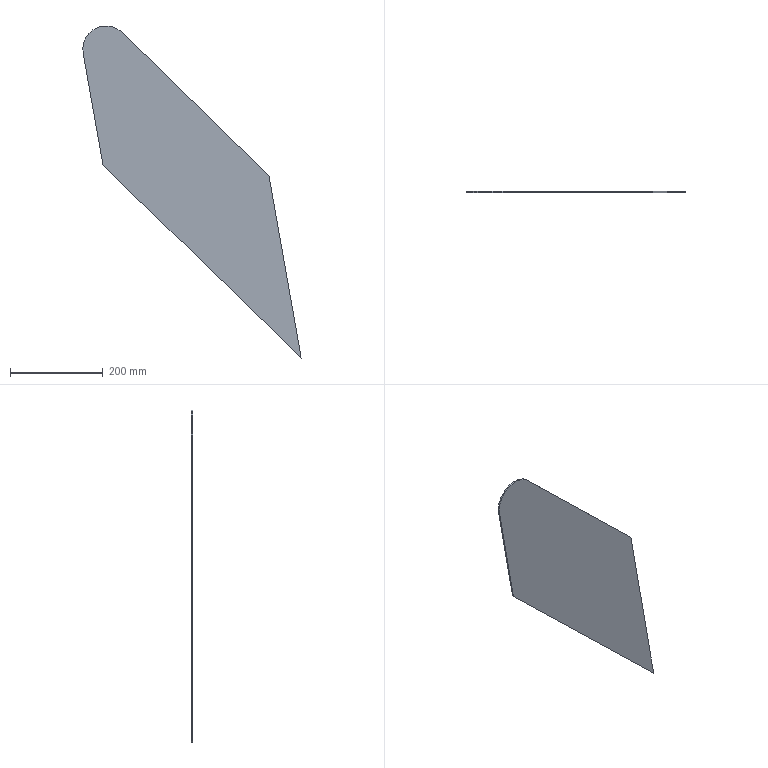Part | STEP file | floating channel side plate 02 | 1 solid | 7 faces | box 470.946 x 3 x 716.27 mm | volume 404515 mm3 | plane 6 | cylinder 1 | commonest cylinder face diameters 100 x1
STEP:
#1=CARTESIAN_POINT('',(0.,0.,0.));
#2=DIRECTION('',(0.,0.,1.));
#3=DIRECTION('',(1.,0.,0.));
#4=AXIS2_PLACEMENT_3D('',#1,#2,#3);
#5=CARTESIAN_POINT('',(1683.637,33.5,379.557));
#6=VERTEX_POINT('',#5);
#7=CARTESIAN_POINT('',(1599.516,33.5,335.038));
#8=VERTEX_POINT('',#7);
#9=CARTESIAN_POINT('',(1648.754,33.5,343.736));
#10=DIRECTION('',(0.,-1.,0.));
#11=DIRECTION('',(0.,0.,-1.));
#12=AXIS2_PLACEMENT_3D('',#9,#10,#11);
#13=CIRCLE('',#12,50.);
#14=CARTESIAN_POINT('',(1648.754,33.5,343.736));
#15=DIRECTION('',(0.,1.,0.));
#16=DIRECTION('',(0.,0.,-1.));
#17=AXIS2_PLACEMENT_3D('',#14,#15,#16);
#18=CYLINDRICAL_SURFACE('',#17,50.);
#19=CARTESIAN_POINT('',(6.283,0.));
#20=DIRECTION('',(-1.,0.));
#21=VECTOR('',#20,1.);
#22=LINE('',#19,#21);
#23=(GEOMETRIC_REPRESENTATION_CONTEXT(2)PARAMETRIC_REPRESENTATION_CONTEXT()REPRESENTATION_CONTEXT('',''));
#24=DEFINITIONAL_REPRESENTATION('',(#22),#23);
#25=PCURVE('',#18,#24);
#26=CARTESIAN_POINT('',(0.,33.5,0.));
#27=DIRECTION('',(0.,-1.,0.));
#28=DIRECTION('',(0.,0.,1.));
#29=AXIS2_PLACEMENT_3D('',#26,#27,#28);
#30=PLANE('',#29);
#31=CARTESIAN_POINT('',(343.736,-1648.754));
#32=DIRECTION('',(-1.,0.));
#33=AXIS2_PLACEMENT_2D('',#31,#32);
#34=CIRCLE('',#33,50.);
#35=(GEOMETRIC_REPRESENTATION_CONTEXT(2)PARAMETRIC_REPRESENTATION_CONTEXT()REPRESENTATION_CONTEXT('',''));
#36=DEFINITIONAL_REPRESENTATION('',(#34),#35);
#37=PCURVE('',#30,#36);
#38=SURFACE_CURVE('',#13,(#25,#37),.PCURVE_S1.);
#39=EDGE_CURVE('',#6,#8,#38,.T.);
#40=ORIENTED_EDGE('',*,*,#39,.F.);
#41=CARTESIAN_POINT('',(1683.637,36.5,379.557));
#42=VERTEX_POINT('',#41);
#43=CARTESIAN_POINT('',(1683.637,33.5,379.557));
#44=DIRECTION('',(0.,-1.,0.));
#45=VECTOR('',#44,1.);
#46=LINE('',#43,#45);
#47=CARTESIAN_POINT('',(3.914,0.));
#48=DIRECTION('',(0.,-1.));
#49=VECTOR('',#48,1.);
#50=LINE('',#47,#49);
#51=(GEOMETRIC_REPRESENTATION_CONTEXT(2)PARAMETRIC_REPRESENTATION_CONTEXT()REPRESENTATION_CONTEXT('',''));
#52=DEFINITIONAL_REPRESENTATION('',(#50),#51);
#53=PCURVE('',#18,#52);
#54=CARTESIAN_POINT('',(2000.11,33.5,71.366));
#55=DIRECTION('',(-0.6977,0.,-0.7164));
#56=DIRECTION('',(0.7164,0.,-0.6977));
#57=AXIS2_PLACEMENT_3D('',#54,#55,#56);
#58=PLANE('',#57);
#59=CARTESIAN_POINT('',(-441.743,0.));
#60=DIRECTION('',(0.,1.));
#61=VECTOR('',#60,1.);
#62=LINE('',#59,#61);
#63=(GEOMETRIC_REPRESENTATION_CONTEXT(2)PARAMETRIC_REPRESENTATION_CONTEXT()REPRESENTATION_CONTEXT('',''));
#64=DEFINITIONAL_REPRESENTATION('',(#62),#63);
#65=PCURVE('',#58,#64);
#66=SURFACE_CURVE('',#46,(#53,#65),.PCURVE_S1.);
#67=EDGE_CURVE('',#42,#6,#66,.T.);
#68=ORIENTED_EDGE('',*,*,#67,.F.);
#69=CARTESIAN_POINT('',(1599.516,36.5,335.038));
#70=VERTEX_POINT('',#69);
#71=CARTESIAN_POINT('',(1648.754,36.5,343.736));
#72=DIRECTION('',(0.,1.,0.));
#73=DIRECTION('',(0.,0.,-1.));
#74=AXIS2_PLACEMENT_3D('',#71,#72,#73);
#75=CIRCLE('',#74,50.);
#76=CARTESIAN_POINT('',(0.,3.));
#77=DIRECTION('',(1.,0.));
#78=VECTOR('',#77,1.);
#79=LINE('',#76,#78);
#80=(GEOMETRIC_REPRESENTATION_CONTEXT(2)PARAMETRIC_REPRESENTATION_CONTEXT()REPRESENTATION_CONTEXT('',''));
#81=DEFINITIONAL_REPRESENTATION('',(#79),#80);
#82=PCURVE('',#18,#81);
#83=CARTESIAN_POINT('',(0.,36.5,0.));
#84=DIRECTION('',(0.,-1.,0.));
#85=DIRECTION('',(0.,0.,1.));
#86=AXIS2_PLACEMENT_3D('',#83,#84,#85);
#87=PLANE('',#86);
#88=CARTESIAN_POINT('',(293.736,-1648.754));
#89=CARTESIAN_POINT('',(293.736,-1562.151));
#90=CARTESIAN_POINT('',(368.736,-1605.452));
#91=CARTESIAN_POINT('',(443.736,-1648.754));
#92=CARTESIAN_POINT('',(368.736,-1692.055));
#93=CARTESIAN_POINT('',(293.736,-1735.356));
#94=CARTESIAN_POINT('',(293.736,-1648.754));
#95=(BOUNDED_CURVE()B_SPLINE_CURVE(2,(#88,#89,#90,#91,#92,#93,#94),.UNSPECIFIED.,.T.,.F.)B_SPLINE_CURVE_WITH_KNOTS((1,2,2,2,2,1),(-2.094,0.,2.094,4.189,6.283,8.378),.UNSPECIFIED.)CURVE()GEOMETRIC_REPRESENTATION_ITEM()RATIONAL_B_SPLINE_CURVE((1.,0.5,1.,0.5,1.,0.5,1.))REPRESENTATION_ITEM(''));
#96=(GEOMETRIC_REPRESENTATION_CONTEXT(2)PARAMETRIC_REPRESENTATION_CONTEXT()REPRESENTATION_CONTEXT('',''));
#97=DEFINITIONAL_REPRESENTATION('',(#95),#96);
#98=PCURVE('',#87,#97);
#99=SURFACE_CURVE('',#75,(#82,#98),.PCURVE_S1.);
#100=EDGE_CURVE('',#70,#42,#99,.T.);
#101=ORIENTED_EDGE('',*,*,#100,.F.);
#102=CARTESIAN_POINT('',(1599.516,33.5,335.038));
#103=DIRECTION('',(0.,1.,0.));
#104=VECTOR('',#103,1.);
#105=LINE('',#102,#104);
#106=CARTESIAN_POINT('',(1.396,0.));
#107=DIRECTION('',(0.,1.));
#108=VECTOR('',#107,1.);
#109=LINE('',#106,#108);
#110=(GEOMETRIC_REPRESENTATION_CONTEXT(2)PARAMETRIC_REPRESENTATION_CONTEXT()REPRESENTATION_CONTEXT('',''));
#111=DEFINITIONAL_REPRESENTATION('',(#109),#110);
#112=PCURVE('',#18,#111);
#113=CARTESIAN_POINT('',(1572.537,33.5,487.751));
#114=DIRECTION('',(0.9848,0.,0.174));
#115=DIRECTION('',(-0.174,0.,0.9848));
#116=AXIS2_PLACEMENT_3D('',#113,#114,#115);
#117=PLANE('',#116);
#118=CARTESIAN_POINT('',(-155.078,0.));
#119=DIRECTION('',(0.,-1.));
#120=VECTOR('',#119,1.);
#121=LINE('',#118,#120);
#122=(GEOMETRIC_REPRESENTATION_CONTEXT(2)PARAMETRIC_REPRESENTATION_CONTEXT()REPRESENTATION_CONTEXT('',''));
#123=DEFINITIONAL_REPRESENTATION('',(#121),#122);
#124=PCURVE('',#117,#123);
#125=SURFACE_CURVE('',#105,(#112,#124),.PCURVE_S1.);
#126=EDGE_CURVE('',#8,#70,#125,.T.);
#127=ORIENTED_EDGE('',*,*,#126,.F.);
#128=EDGE_LOOP('',(#40,#68,#101,#127));
#129=FACE_BOUND('',#128,.T.);
#130=ADVANCED_FACE('',(#129),#18,.T.);
#131=CARTESIAN_POINT('',(1642.126,36.5,93.851));
#132=VERTEX_POINT('',#131);
#133=CARTESIAN_POINT('',(1572.537,36.5,487.751));
#134=DIRECTION('',(0.174,0.,-0.9848));
#135=VECTOR('',#134,1.);
#136=LINE('',#133,#135);
#137=CARTESIAN_POINT('',(487.751,-1572.537));
#138=DIRECTION('',(-0.9848,-0.174));
#139=VECTOR('',#138,1.);
#140=LINE('',#137,#139);
#141=(GEOMETRIC_REPRESENTATION_CONTEXT(2)PARAMETRIC_REPRESENTATION_CONTEXT()REPRESENTATION_CONTEXT('',''));
#142=DEFINITIONAL_REPRESENTATION('',(#140),#141);
#143=PCURVE('',#87,#142);
#144=CARTESIAN_POINT('',(0.,-3.));
#145=DIRECTION('',(-1.,0.));
#146=VECTOR('',#145,1.);
#147=LINE('',#144,#146);
#148=(GEOMETRIC_REPRESENTATION_CONTEXT(2)PARAMETRIC_REPRESENTATION_CONTEXT()REPRESENTATION_CONTEXT('',''));
#149=DEFINITIONAL_REPRESENTATION('',(#147),#148);
#150=PCURVE('',#117,#149);
#151=SURFACE_CURVE('',#136,(#143,#150),.PCURVE_S1.);
#152=EDGE_CURVE('',#70,#132,#151,.T.);
#153=ORIENTED_EDGE('',*,*,#152,.F.);
#154=ORIENTED_EDGE('',*,*,#100,.T.);
#155=CARTESIAN_POINT('',(2000.11,36.5,71.366));
#156=VERTEX_POINT('',#155);
#157=CARTESIAN_POINT('',(2000.11,36.5,71.366));
#158=DIRECTION('',(-0.7164,0.,0.6977));
#159=VECTOR('',#158,1.);
#160=LINE('',#157,#159);
#161=CARTESIAN_POINT('',(71.366,-2000.11));
#162=DIRECTION('',(0.6977,0.7164));
#163=VECTOR('',#162,1.);
#164=LINE('',#161,#163);
#165=(GEOMETRIC_REPRESENTATION_CONTEXT(2)PARAMETRIC_REPRESENTATION_CONTEXT()REPRESENTATION_CONTEXT('',''));
#166=DEFINITIONAL_REPRESENTATION('',(#164),#165);
#167=PCURVE('',#87,#166);
#168=CARTESIAN_POINT('',(0.,-3.));
#169=DIRECTION('',(-1.,0.));
#170=VECTOR('',#169,1.);
#171=LINE('',#168,#170);
#172=(GEOMETRIC_REPRESENTATION_CONTEXT(2)PARAMETRIC_REPRESENTATION_CONTEXT()REPRESENTATION_CONTEXT('',''));
#173=DEFINITIONAL_REPRESENTATION('',(#171),#172);
#174=PCURVE('',#58,#173);
#175=SURFACE_CURVE('',#160,(#167,#174),.PCURVE_S1.);
#176=EDGE_CURVE('',#156,#42,#175,.T.);
#177=ORIENTED_EDGE('',*,*,#176,.F.);
#178=CARTESIAN_POINT('',(2069.699,36.5,-322.534));
#179=VERTEX_POINT('',#178);
#180=CARTESIAN_POINT('',(2069.699,36.5,-322.534));
#181=DIRECTION('',(-0.174,0.,0.9848));
#182=VECTOR('',#181,1.);
#183=LINE('',#180,#182);
#184=CARTESIAN_POINT('',(-322.534,-2069.699));
#185=DIRECTION('',(0.9848,0.174));
#186=VECTOR('',#185,1.);
#187=LINE('',#184,#186);
#188=(GEOMETRIC_REPRESENTATION_CONTEXT(2)PARAMETRIC_REPRESENTATION_CONTEXT()REPRESENTATION_CONTEXT('',''));
#189=DEFINITIONAL_REPRESENTATION('',(#187),#188);
#190=PCURVE('',#87,#189);
#191=CARTESIAN_POINT('',(2069.699,33.5,-322.534));
#192=DIRECTION('',(-0.9848,0.,-0.174));
#193=DIRECTION('',(0.174,0.,-0.9848));
#194=AXIS2_PLACEMENT_3D('',#191,#192,#193);
#195=PLANE('',#194);
#196=CARTESIAN_POINT('',(0.,-3.));
#197=DIRECTION('',(-1.,0.));
#198=VECTOR('',#197,1.);
#199=LINE('',#196,#198);
#200=(GEOMETRIC_REPRESENTATION_CONTEXT(2)PARAMETRIC_REPRESENTATION_CONTEXT()REPRESENTATION_CONTEXT('',''));
#201=DEFINITIONAL_REPRESENTATION('',(#199),#200);
#202=PCURVE('',#195,#201);
#203=SURFACE_CURVE('',#183,(#190,#202),.PCURVE_S1.);
#204=EDGE_CURVE('',#179,#156,#203,.T.);
#205=ORIENTED_EDGE('',*,*,#204,.F.);
#206=CARTESIAN_POINT('',(1642.126,36.5,93.851));
#207=DIRECTION('',(0.7164,0.,-0.6977));
#208=VECTOR('',#207,1.);
#209=LINE('',#206,#208);
#210=CARTESIAN_POINT('',(93.851,-1642.126));
#211=DIRECTION('',(-0.6977,-0.7164));
#212=VECTOR('',#211,1.);
#213=LINE('',#210,#212);
#214=(GEOMETRIC_REPRESENTATION_CONTEXT(2)PARAMETRIC_REPRESENTATION_CONTEXT()REPRESENTATION_CONTEXT('',''));
#215=DEFINITIONAL_REPRESENTATION('',(#213),#214);
#216=PCURVE('',#87,#215);
#217=CARTESIAN_POINT('',(1642.126,33.5,93.851));
#218=DIRECTION('',(0.6977,0.,0.7164));
#219=DIRECTION('',(-0.7164,0.,0.6977));
#220=AXIS2_PLACEMENT_3D('',#217,#218,#219);
#221=PLANE('',#220);
#222=CARTESIAN_POINT('',(0.,-3.));
#223=DIRECTION('',(-1.,0.));
#224=VECTOR('',#223,1.);
#225=LINE('',#222,#224);
#226=(GEOMETRIC_REPRESENTATION_CONTEXT(2)PARAMETRIC_REPRESENTATION_CONTEXT()REPRESENTATION_CONTEXT('',''));
#227=DEFINITIONAL_REPRESENTATION('',(#225),#226);
#228=PCURVE('',#221,#227);
#229=SURFACE_CURVE('',#209,(#216,#228),.PCURVE_S1.);
#230=EDGE_CURVE('',#132,#179,#229,.T.);
#231=ORIENTED_EDGE('',*,*,#230,.F.);
#232=EDGE_LOOP('',(#153,#154,#177,#205,#231));
#233=FACE_BOUND('',#232,.T.);
#234=ADVANCED_FACE('',(#233),#87,.F.);
#235=CARTESIAN_POINT('',(2000.11,33.5,71.366));
#236=VERTEX_POINT('',#235);
#237=CARTESIAN_POINT('',(2000.11,33.5,71.366));
#238=DIRECTION('',(-0.7164,0.,0.6977));
#239=VECTOR('',#238,1.);
#240=LINE('',#237,#239);
#241=CARTESIAN_POINT('',(71.366,-2000.11));
#242=DIRECTION('',(0.6977,0.7164));
#243=VECTOR('',#242,1.);
#244=LINE('',#241,#243);
#245=(GEOMETRIC_REPRESENTATION_CONTEXT(2)PARAMETRIC_REPRESENTATION_CONTEXT()REPRESENTATION_CONTEXT('',''));
#246=DEFINITIONAL_REPRESENTATION('',(#244),#245);
#247=PCURVE('',#30,#246);
#248=CARTESIAN_POINT('',(0.,0.));
#249=DIRECTION('',(-1.,0.));
#250=VECTOR('',#249,1.);
#251=LINE('',#248,#250);
#252=(GEOMETRIC_REPRESENTATION_CONTEXT(2)PARAMETRIC_REPRESENTATION_CONTEXT()REPRESENTATION_CONTEXT('',''));
#253=DEFINITIONAL_REPRESENTATION('',(#251),#252);
#254=PCURVE('',#58,#253);
#255=SURFACE_CURVE('',#240,(#247,#254),.PCURVE_S1.);
#256=EDGE_CURVE('',#236,#6,#255,.T.);
#257=ORIENTED_EDGE('',*,*,#256,.T.);
#258=ORIENTED_EDGE('',*,*,#39,.T.);
#259=CARTESIAN_POINT('',(1642.126,33.5,93.851));
#260=VERTEX_POINT('',#259);
#261=CARTESIAN_POINT('',(1572.537,33.5,487.751));
#262=DIRECTION('',(0.174,0.,-0.9848));
#263=VECTOR('',#262,1.);
#264=LINE('',#261,#263);
#265=CARTESIAN_POINT('',(487.751,-1572.537));
#266=DIRECTION('',(-0.9848,-0.174));
#267=VECTOR('',#266,1.);
#268=LINE('',#265,#267);
#269=(GEOMETRIC_REPRESENTATION_CONTEXT(2)PARAMETRIC_REPRESENTATION_CONTEXT()REPRESENTATION_CONTEXT('',''));
#270=DEFINITIONAL_REPRESENTATION('',(#268),#269);
#271=PCURVE('',#30,#270);
#272=CARTESIAN_POINT('',(0.,0.));
#273=DIRECTION('',(-1.,0.));
#274=VECTOR('',#273,1.);
#275=LINE('',#272,#274);
#276=(GEOMETRIC_REPRESENTATION_CONTEXT(2)PARAMETRIC_REPRESENTATION_CONTEXT()REPRESENTATION_CONTEXT('',''));
#277=DEFINITIONAL_REPRESENTATION('',(#275),#276);
#278=PCURVE('',#117,#277);
#279=SURFACE_CURVE('',#264,(#271,#278),.PCURVE_S1.);
#280=EDGE_CURVE('',#8,#260,#279,.T.);
#281=ORIENTED_EDGE('',*,*,#280,.T.);
#282=CARTESIAN_POINT('',(2069.699,33.5,-322.534));
#283=VERTEX_POINT('',#282);
#284=CARTESIAN_POINT('',(1642.126,33.5,93.851));
#285=DIRECTION('',(0.7164,0.,-0.6977));
#286=VECTOR('',#285,1.);
#287=LINE('',#284,#286);
#288=CARTESIAN_POINT('',(93.851,-1642.126));
#289=DIRECTION('',(-0.6977,-0.7164));
#290=VECTOR('',#289,1.);
#291=LINE('',#288,#290);
#292=(GEOMETRIC_REPRESENTATION_CONTEXT(2)PARAMETRIC_REPRESENTATION_CONTEXT()REPRESENTATION_CONTEXT('',''));
#293=DEFINITIONAL_REPRESENTATION('',(#291),#292);
#294=PCURVE('',#30,#293);
#295=CARTESIAN_POINT('',(0.,0.));
#296=DIRECTION('',(-1.,0.));
#297=VECTOR('',#296,1.);
#298=LINE('',#295,#297);
#299=(GEOMETRIC_REPRESENTATION_CONTEXT(2)PARAMETRIC_REPRESENTATION_CONTEXT()REPRESENTATION_CONTEXT('',''));
#300=DEFINITIONAL_REPRESENTATION('',(#298),#299);
#301=PCURVE('',#221,#300);
#302=SURFACE_CURVE('',#287,(#294,#301),.PCURVE_S1.);
#303=EDGE_CURVE('',#260,#283,#302,.T.);
#304=ORIENTED_EDGE('',*,*,#303,.T.);
#305=CARTESIAN_POINT('',(2069.699,33.5,-322.534));
#306=DIRECTION('',(-0.174,0.,0.9848));
#307=VECTOR('',#306,1.);
#308=LINE('',#305,#307);
#309=CARTESIAN_POINT('',(-322.534,-2069.699));
#310=DIRECTION('',(0.9848,0.174));
#311=VECTOR('',#310,1.);
#312=LINE('',#309,#311);
#313=(GEOMETRIC_REPRESENTATION_CONTEXT(2)PARAMETRIC_REPRESENTATION_CONTEXT()REPRESENTATION_CONTEXT('',''));
#314=DEFINITIONAL_REPRESENTATION('',(#312),#313);
#315=PCURVE('',#30,#314);
#316=CARTESIAN_POINT('',(0.,0.));
#317=DIRECTION('',(-1.,0.));
#318=VECTOR('',#317,1.);
#319=LINE('',#316,#318);
#320=(GEOMETRIC_REPRESENTATION_CONTEXT(2)PARAMETRIC_REPRESENTATION_CONTEXT()REPRESENTATION_CONTEXT('',''));
#321=DEFINITIONAL_REPRESENTATION('',(#319),#320);
#322=PCURVE('',#195,#321);
#323=SURFACE_CURVE('',#308,(#315,#322),.PCURVE_S1.);
#324=EDGE_CURVE('',#283,#236,#323,.T.);
#325=ORIENTED_EDGE('',*,*,#324,.T.);
#326=EDGE_LOOP('',(#257,#258,#281,#304,#325));
#327=FACE_BOUND('',#326,.T.);
#328=ADVANCED_FACE('',(#327),#30,.T.);
#329=ORIENTED_EDGE('',*,*,#230,.T.);
#330=CARTESIAN_POINT('',(2069.699,33.5,-322.534));
#331=DIRECTION('',(0.,1.,0.));
#332=VECTOR('',#331,1.);
#333=LINE('',#330,#332);
#334=CARTESIAN_POINT('',(-596.821,0.));
#335=DIRECTION('',(0.,-1.));
#336=VECTOR('',#335,1.);
#337=LINE('',#334,#336);
#338=(GEOMETRIC_REPRESENTATION_CONTEXT(2)PARAMETRIC_REPRESENTATION_CONTEXT()REPRESENTATION_CONTEXT('',''));
#339=DEFINITIONAL_REPRESENTATION('',(#337),#338);
#340=PCURVE('',#221,#339);
#341=CARTESIAN_POINT('',(0.,0.));
#342=DIRECTION('',(0.,-1.));
#343=VECTOR('',#342,1.);
#344=LINE('',#341,#343);
#345=(GEOMETRIC_REPRESENTATION_CONTEXT(2)PARAMETRIC_REPRESENTATION_CONTEXT()REPRESENTATION_CONTEXT('',''));
#346=DEFINITIONAL_REPRESENTATION('',(#344),#345);
#347=PCURVE('',#195,#346);
#348=SURFACE_CURVE('',#333,(#340,#347),.PCURVE_S1.);
#349=EDGE_CURVE('',#283,#179,#348,.T.);
#350=ORIENTED_EDGE('',*,*,#349,.F.);
#351=ORIENTED_EDGE('',*,*,#303,.F.);
#352=CARTESIAN_POINT('',(1642.126,33.5,93.851));
#353=DIRECTION('',(0.,1.,0.));
#354=VECTOR('',#353,1.);
#355=LINE('',#352,#354);
#356=CARTESIAN_POINT('',(0.,0.));
#357=DIRECTION('',(0.,-1.));
#358=VECTOR('',#357,1.);
#359=LINE('',#356,#358);
#360=(GEOMETRIC_REPRESENTATION_CONTEXT(2)PARAMETRIC_REPRESENTATION_CONTEXT()REPRESENTATION_CONTEXT('',''));
#361=DEFINITIONAL_REPRESENTATION('',(#359),#360);
#362=PCURVE('',#221,#361);
#363=CARTESIAN_POINT('',(-400.,0.));
#364=DIRECTION('',(0.,-1.));
#365=VECTOR('',#364,1.);
#366=LINE('',#363,#365);
#367=(GEOMETRIC_REPRESENTATION_CONTEXT(2)PARAMETRIC_REPRESENTATION_CONTEXT()REPRESENTATION_CONTEXT('',''));
#368=DEFINITIONAL_REPRESENTATION('',(#366),#367);
#369=PCURVE('',#117,#368);
#370=SURFACE_CURVE('',#355,(#362,#369),.PCURVE_S1.);
#371=EDGE_CURVE('',#260,#132,#370,.T.);
#372=ORIENTED_EDGE('',*,*,#371,.T.);
#373=EDGE_LOOP('',(#329,#350,#351,#372));
#374=FACE_BOUND('',#373,.T.);
#375=ADVANCED_FACE('',(#374),#221,.F.);
#376=ORIENTED_EDGE('',*,*,#280,.F.);
#377=ORIENTED_EDGE('',*,*,#126,.T.);
#378=ORIENTED_EDGE('',*,*,#152,.T.);
#379=ORIENTED_EDGE('',*,*,#371,.F.);
#380=EDGE_LOOP('',(#376,#377,#378,#379));
#381=FACE_BOUND('',#380,.T.);
#382=ADVANCED_FACE('',(#381),#117,.F.);
#383=ORIENTED_EDGE('',*,*,#176,.T.);
#384=ORIENTED_EDGE('',*,*,#67,.T.);
#385=ORIENTED_EDGE('',*,*,#256,.F.);
#386=CARTESIAN_POINT('',(2000.11,33.5,71.366));
#387=DIRECTION('',(0.,1.,0.));
#388=VECTOR('',#387,1.);
#389=LINE('',#386,#388);
#390=CARTESIAN_POINT('',(0.,0.));
#391=DIRECTION('',(0.,-1.));
#392=VECTOR('',#391,1.);
#393=LINE('',#390,#392);
#394=(GEOMETRIC_REPRESENTATION_CONTEXT(2)PARAMETRIC_REPRESENTATION_CONTEXT()REPRESENTATION_CONTEXT('',''));
#395=DEFINITIONAL_REPRESENTATION('',(#393),#394);
#396=PCURVE('',#58,#395);
#397=CARTESIAN_POINT('',(-400.,0.));
#398=DIRECTION('',(0.,-1.));
#399=VECTOR('',#398,1.);
#400=LINE('',#397,#399);
#401=(GEOMETRIC_REPRESENTATION_CONTEXT(2)PARAMETRIC_REPRESENTATION_CONTEXT()REPRESENTATION_CONTEXT('',''));
#402=DEFINITIONAL_REPRESENTATION('',(#400),#401);
#403=PCURVE('',#195,#402);
#404=SURFACE_CURVE('',#389,(#396,#403),.PCURVE_S1.);
#405=EDGE_CURVE('',#236,#156,#404,.T.);
#406=ORIENTED_EDGE('',*,*,#405,.T.);
#407=EDGE_LOOP('',(#383,#384,#385,#406));
#408=FACE_BOUND('',#407,.T.);
#409=ADVANCED_FACE('',(#408),#58,.F.);
#410=ORIENTED_EDGE('',*,*,#204,.T.);
#411=ORIENTED_EDGE('',*,*,#405,.F.);
#412=ORIENTED_EDGE('',*,*,#324,.F.);
#413=ORIENTED_EDGE('',*,*,#349,.T.);
#414=EDGE_LOOP('',(#410,#411,#412,#413));
#415=FACE_BOUND('',#414,.T.);
#416=ADVANCED_FACE('',(#415),#195,.F.);
#417=CLOSED_SHELL('',(#130,#234,#328,#375,#382,#409,#416));
#418=MANIFOLD_SOLID_BREP('',#417);
#419=(LENGTH_UNIT()NAMED_UNIT(*)SI_UNIT(.MILLI.,.METRE.));
#420=UNCERTAINTY_MEASURE_WITH_UNIT(LENGTH_MEASURE(0.0000001),#419,'','');
#421=(NAMED_UNIT(*)PLANE_ANGLE_UNIT()SI_UNIT($,.RADIAN.));
#422=(NAMED_UNIT(*)SI_UNIT($,.STERADIAN.)SOLID_ANGLE_UNIT());
#423=(GEOMETRIC_REPRESENTATION_CONTEXT(3)GLOBAL_UNCERTAINTY_ASSIGNED_CONTEXT((#420))GLOBAL_UNIT_ASSIGNED_CONTEXT((#419,#421,#422))REPRESENTATION_CONTEXT('',''));
#424=ADVANCED_BREP_SHAPE_REPRESENTATION('',(#4,#418),#423);